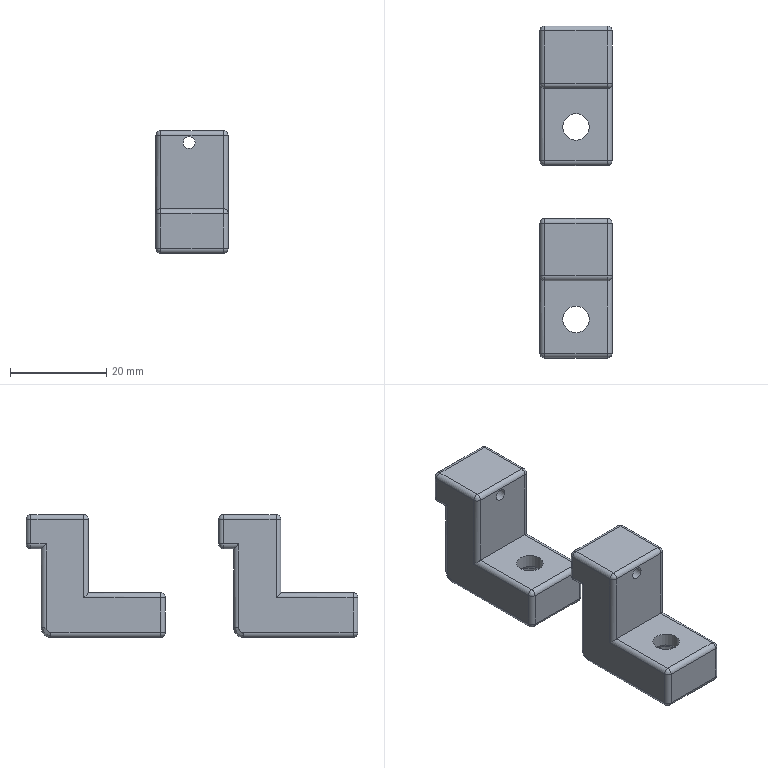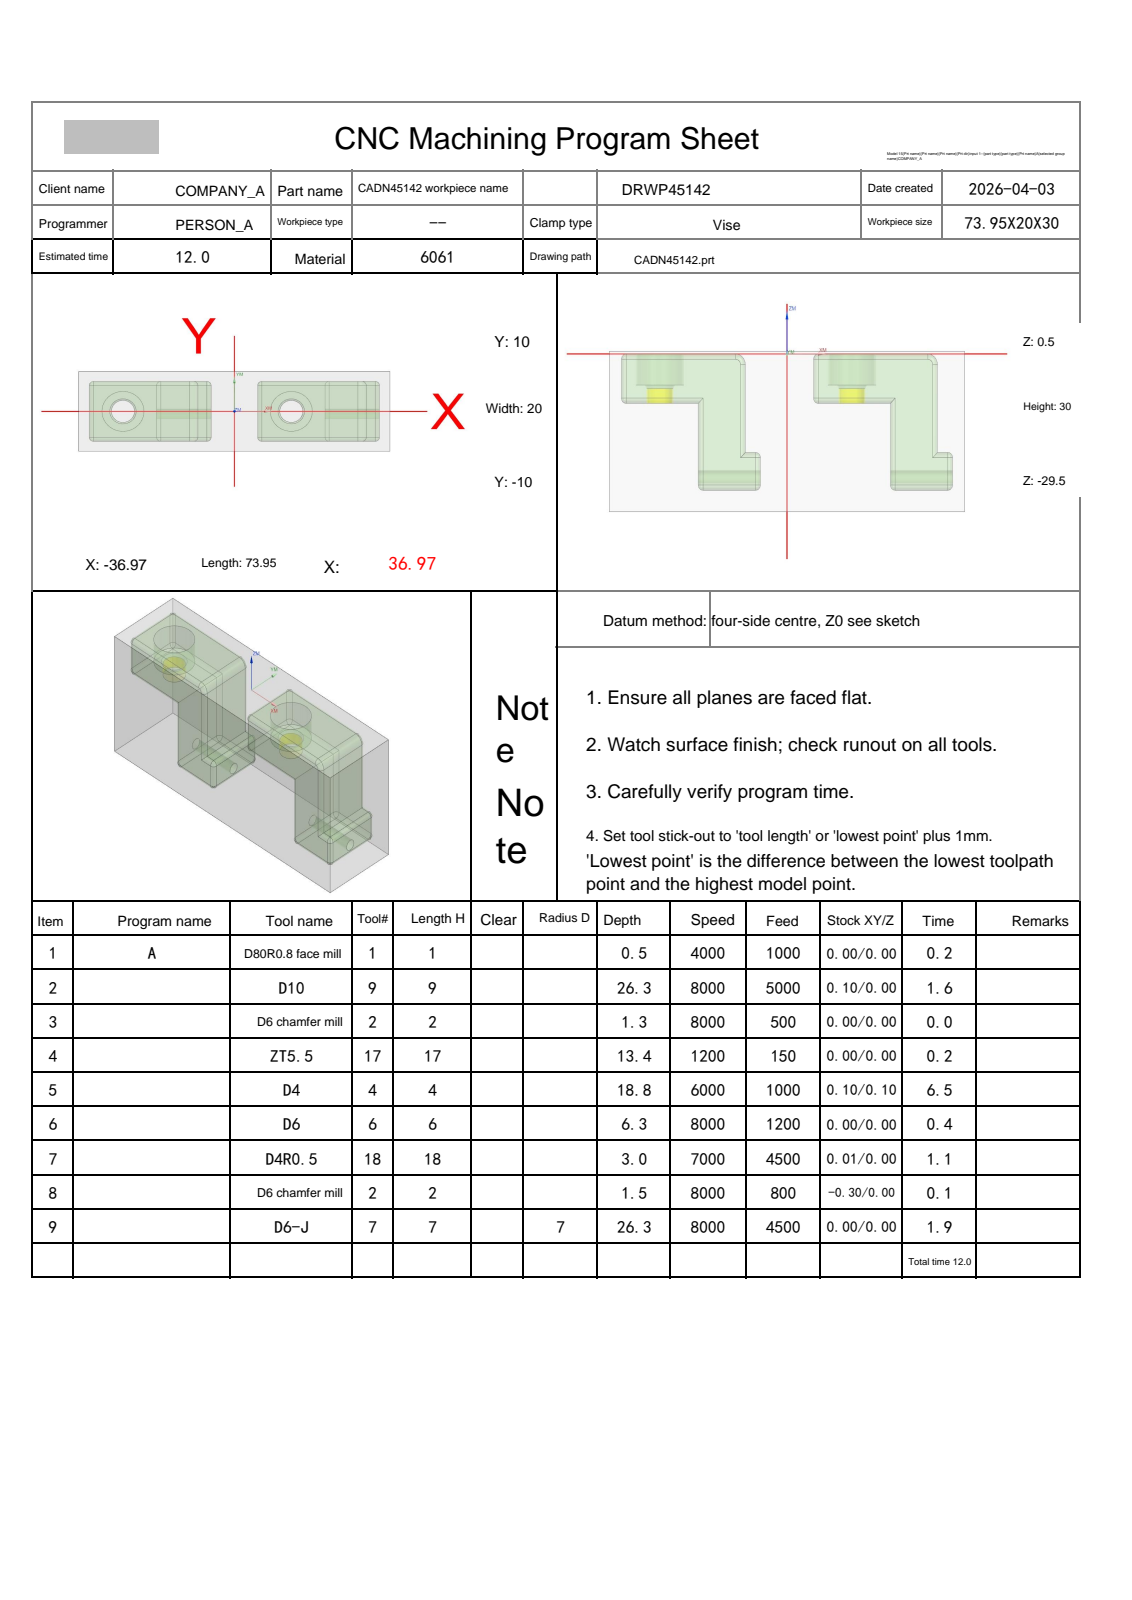NC program | NX | posted by the shop | part box 15 x 68.95 x 25.5 mm
Lines 4665 to 6074 of 6074:
N9 T07 M06
(D6-J  D=6. R=0. H=07 ce=0.00 di=0.00)
G00 G90 G54 X-34.389 Y11.516 M03 S8000
G43 H07 Z5.5
M08
Z-8.207
G01 Z-9.207 F1000.
G41 D07
X-34.371 Y11.317
G03 X-33.475 Y10.5 I.896 J.083
G01 X-9.675
X-9.386 Y10.489
G02 X-5.778 Y7.404 I-.289 J-3.99
X-5.675 Y6.5 I-3.896 J-.904
G01 X-5.674 Y-6.5
G02 X-5.736 Y-7.2 I-4. J0.0
X-9.674 Y-10.5 I-3.938 J.7
G01 X-33.475
G02 X-37.475 Y-6.5 I0.0 J4.
G01 Y6.5
G02 X-33.475 Y10.5 I4. J0.0
G03 X-32.575 Y11.4 I0.0 J.9
G01 G40 Y11.6
Z-8.207
G00 X-34.389 Y11.516
Z-17.413
G01 Z-18.413
G41 D07
X-34.371 Y11.317
G03 X-33.475 Y10.5 I.896 J.083
G01 X-9.675
G02 X-5.675 Y6.5 I0.0 J-4.
G01 X-5.674 Y-6.5
G02 X-9.674 Y-10.5 I-4. J0.0
G01 X-33.475
G02 X-37.475 Y-6.5 I0.0 J4.
G01 Y6.5
G02 X-33.475 Y10.5 I4. J0.0
G03 X-32.575 Y11.4 I0.0 J.9
G01 G40 Y11.6
Z-17.413
G00 Z5.5
X5.611 Y11.516
Z-8.207
G01 Z-9.207
G41 D07
X5.629 Y11.317
G03 X6.525 Y10.5 I.896 J.083
G01 X30.325
G02 X34.273 Y7.147 I0.0 J-4.
X34.325 Y6.5 I-3.947 J-.647
G01 X34.326 Y-6.5
G02 X30.326 Y-10.5 I-4. J0.0
G01 X6.525
G02 X2.525 Y-6.5 I0.0 J4.
G01 Y6.5
G02 X6.525 Y10.5 I4. J0.0
G03 X7.425 Y11.4 I0.0 J.9
G01 G40 Y11.6
Z-8.207
G00 X5.611 Y11.516
Z-17.413
G01 Z-18.413
G41 D07
X5.629 Y11.317
G03 X6.525 Y10.5 I.896 J.083
G01 X30.325
G02 X34.325 Y6.5 I0.0 J-4.
G01 X34.326 Y-6.5
G02 X30.326 Y-10.5 I-4. J0.0
G01 X6.525
G02 X2.525 Y-6.5 I0.0 J4.
G01 Y6.5
G02 X6.525 Y10.5 I4. J0.0
G03 X7.425 Y11.4 I0.0 J.9
G01 G40 Y11.6
Z-17.413
G00 Z5.5
G00 G90 X32.554 Y11.209 M03 S7000
Z10.5
Z-17.921
G01 Z-18.421 F4500.
G03 X32.372 Y10.575 I1.018 J-.635
X32.824 Y9.636 I1.2 J0.0
G01 X33.475
G02 X36.611 Y6.5 I0.0 J-3.136
G01 Y-6.5
G02 X33.475 Y-9.636 I-3.136 J0.0
G01 X32.825
X32.789 Y-9.664 Z-18.425
X33.475
G03 X36.639 Y-6.5 I0.0 J3.164
G01 Y6.5
G03 X33.475 Y9.664 I-3.164 J0.0
G01 X32.788
X32.758 Y9.688 Z-18.429
X33.475
G02 X36.663 Y6.5 I0.0 J-3.188
G01 Y-6.5
G02 X33.475 Y-9.688 I-3.188 J0.0
G01 X32.758
X32.73 Y-9.709 Z-18.433
X33.475
G03 X36.684 Y-6.5 I0.0 J3.209
G01 Y6.5
G03 X33.475 Y9.709 I-3.209 J0.0
G01 X32.73
X32.705 Y9.728 Z-18.437
X33.475
G02 X36.703 Y6.5 I0.0 J-3.228
G01 Y-6.5
G02 X33.475 Y-9.728 I-3.228 J0.0
G01 X32.705
X32.682 Y-9.745 Z-18.441
X33.475
G03 X36.72 Y-6.5 I0.0 J3.245
G01 Y6.5
G03 X33.475 Y9.745 I-3.245 J0.0
G01 X32.681
X32.659 Y9.761 Z-18.445
X33.475
G02 X36.736 Y6.5 I0.0 J-3.261
G01 Y-6.5
G02 X33.475 Y-9.761 I-3.261 J0.0
G01 X32.66
X32.638 Y-9.776 Z-18.449
X33.475
G03 X36.751 Y-6.5 I0.0 J3.277
G01 Y6.5
G03 X33.475 Y9.776 I-3.277 J0.0
G01 X32.637
X32.616 Y9.791 Z-18.454
X33.475
G02 X36.766 Y6.5 I0.0 J-3.292
G01 Y-6.5
G02 X33.475 Y-9.791 I-3.292 J0.0
G01 X32.616
X32.594 Y-9.807 Z-18.458
X33.475
G03 X36.782 Y-6.5 I0.0 J3.307
G01 Y6.5
G03 X33.475 Y9.807 I-3.307 J0.0
G01 X32.594
X32.574 Y9.82 Z-18.463
X33.475
G02 X36.795 Y6.5 I0.0 J-3.32
G01 Y-6.5
G02 X33.475 Y-9.82 I-3.32 J0.0
G01 X32.574
Z-18.468
X33.475
G03 X36.795 Y-6.5 I0.0 J3.32
G01 Y6.5
G03 X33.475 Y9.82 I-3.32 J0.0
G01 X32.574
X32.528 Y9.851 Z-18.473
X33.475
G02 X36.826 Y6.5 I0.0 J-3.351
G01 Y-6.5
G02 X33.475 Y-9.851 I-3.351 J0.0
G01 X32.528
X32.518 Y-9.858 Z-18.479
X33.475
G03 X36.833 Y-6.5 I0.0 J3.358
G01 Y6.5
G03 X33.475 Y9.858 I-3.358 J0.0
G01 X32.517
Z-18.484
X33.475
G02 X36.833 Y6.5 I0.0 J-3.358
G01 Y-6.5
G02 X33.475 Y-9.858 I-3.358 J0.0
G01 X32.518
X32.46 Y-9.895 Z-18.49
X33.475
G03 X36.869 Y-6.5 I0.0 J3.395
G01 Y6.5
G03 X33.475 Y9.895 I-3.395 J0.0
G01 X32.46
X32.437 Y9.909 Z-18.496
X33.475
G02 X36.884 Y6.5 I0.0 J-3.409
G01 Y-6.5
G02 X33.475 Y-9.909 I-3.409 J0.0
G01 X32.438
X32.415 Y-9.923 Z-18.502
X33.475
G03 X36.898 Y-6.5 I0.0 J3.423
G01 Y6.5
G03 X33.475 Y9.923 I-3.423 J0.0
G01 X32.414
X32.391 Y9.937 Z-18.509
X33.475
G02 X36.912 Y6.5 I0.0 J-3.437
G01 Y-6.5
G02 X33.475 Y-9.937 I-3.437 J0.0
G01 X32.392
X32.368 Y-9.951 Z-18.516
X33.475
G03 X36.926 Y-6.5 I0.0 J3.451
G01 Y6.5
G03 X33.475 Y9.951 I-3.451 J0.0
G01 X32.368
X32.345 Y9.964 Z-18.522
X33.475
G02 X36.939 Y6.5 I0.0 J-3.464
G01 Y-6.5
G02 X33.475 Y-9.964 I-3.464 J0.0
G01 X32.345
X32.322 Y-9.978 Z-18.529
X33.475
G03 X36.953 Y-6.5 I0.0 J3.478
G01 Y6.5
G03 X33.475 Y9.978 I-3.478 J0.0
G01 X32.321
X32.298 Y9.991 Z-18.537
X33.475
G02 X36.966 Y6.5 I0.0 J-3.491
G01 Y-6.5
G02 X33.475 Y-9.991 I-3.491 J0.0
G01 X32.298
X32.274 Y-10.005 Z-18.544
X33.475
G03 X36.98 Y-6.5 I0.0 J3.505
G01 Y6.5
G03 X33.475 Y10.005 I-3.505 J0.0
G01 X32.274
X32.25 Y10.018 Z-18.552
X33.475
G02 X36.993 Y6.5 I0.0 J-3.518
G01 Y-6.5
G02 X33.475 Y-10.018 I-3.518 J0.0
G01 X32.25
X32.226 Y-10.031 Z-18.56
X33.475
G03 X37.006 Y-6.5 I0.0 J3.531
G01 Y6.5
G03 X33.475 Y10.031 I-3.531 J0.0
G01 X32.226
X32.202 Y10.044 Z-18.568
X33.475
G02 X37.019 Y6.5 I0.0 J-3.544
G01 Y-6.5
G02 X33.475 Y-10.044 I-3.544 J0.0
G01 X32.202
X32.178 Y-10.057 Z-18.576
X33.475
G03 X37.032 Y-6.5 I0.0 J3.557
G01 Y6.5
G03 X33.475 Y10.057 I-3.557 J0.0
G01 X32.177
X32.153 Y10.069 Z-18.584
X33.475
G02 X37.044 Y6.5 I0.0 J-3.569
G01 Y-6.5
G02 X33.475 Y-10.069 I-3.569 J0.0
G01 X32.153
X32.128 Y-10.082 Z-18.593
X33.475
G03 X37.057 Y-6.5 I0.0 J3.582
G01 Y6.5
G03 X33.475 Y10.082 I-3.582 J0.0
G01 X32.128
X32.103 Y10.094 Z-18.602
X33.475
G02 X37.069 Y6.5 I0.0 J-3.594
G01 Y-6.5
G02 X33.475 Y-10.094 I-3.594 J0.0
G01 X32.104
X32.079 Y-10.106 Z-18.611
X33.475
G03 X37.081 Y-6.5 I0.0 J3.607
G01 Y6.5
G03 X33.475 Y10.106 I-3.607 J0.0
G01 X32.078
X32.053 Y10.119 Z-18.62
X33.475
G02 X37.093 Y6.5 I0.0 J-3.619
G01 Y-6.5
G02 X33.475 Y-10.119 I-3.619 J0.0
G01 X32.054
X32.028 Y-10.131 Z-18.629
X33.475
G03 X37.105 Y-6.5 I0.0 J3.631
G01 Y6.5
G03 X33.475 Y10.131 I-3.631 J0.0
G01 X32.028
X32.003 Y10.142 Z-18.639
X33.475
G02 X37.117 Y6.5 I0.0 J-3.642
G01 Y-6.5
G02 X33.475 Y-10.142 I-3.642 J0.0
G01 X32.003
X31.977 Y-10.154 Z-18.648
X33.475
G03 X37.129 Y-6.5 I0.0 J3.654
G01 Y6.5
G03 X33.475 Y10.154 I-3.654 J0.0
G01 X31.977
X31.951 Y10.165 Z-18.658
X33.475
G02 X37.14 Y6.5 I0.0 J-3.666
G01 Y-6.5
G02 X33.475 Y-10.165 I-3.666 J0.0
G01 X31.952
X31.926 Y-10.177 Z-18.668
X33.475
G03 X37.152 Y-6.5 I0.0 J3.677
G01 Y6.5
G03 X33.475 Y10.177 I-3.677 J0.0
G01 X31.925
X31.9 Y10.188 Z-18.678
X33.475
G02 X37.163 Y6.5 I0.0 J-3.688
G01 Y-6.5
G02 X33.475 Y-10.188 I-3.688 J0.0
G01 X31.9
X31.874 Y-10.199 Z-18.689
X33.475
G03 X37.174 Y-6.5 I0.0 J3.699
G01 Y6.5
G03 X33.475 Y10.199 I-3.699 J0.0
G01 X31.873
X31.847 Y10.21 Z-18.699
X33.475
G02 X37.185 Y6.5 I0.0 J-3.71
G01 Y-6.5
G02 X33.475 Y-10.21 I-3.71 J0.0
G01 X31.848
X31.821 Y-10.221 Z-18.71
X33.475
G03 X37.195 Y-6.5 I0.0 J3.721
G01 Y6.5
G03 X33.475 Y10.221 I-3.721 J0.0
G01 X31.821
X31.794 Y10.231 Z-18.72
X33.475
G02 X37.206 Y6.5 I0.0 J-3.731
G01 Y-6.5
G02 X33.475 Y-10.231 I-3.731 J0.0
G01 X31.795
X31.768 Y-10.242 Z-18.731
X33.475
G03 X37.216 Y-6.5 I0.0 J3.742
G01 Y6.5
G03 X33.475 Y10.242 I-3.742 J0.0
G01 X31.768
X31.741 Y10.252 Z-18.743
X33.475
G02 X37.227 Y6.5 I0.0 J-3.752
G01 Y-6.5
G02 X33.475 Y-10.252 I-3.752 J0.0
G01 X31.741
X31.714 Y-10.262 Z-18.754
X33.475
G03 X37.237 Y-6.5 I0.0 J3.762
G01 Y6.5
G03 X33.475 Y10.262 I-3.762 J0.0
G01 X31.714
X31.687 Y10.272 Z-18.765
X33.475
G02 X37.247 Y6.5 I0.0 J-3.772
G01 Y-6.5
G02 X33.475 Y-10.272 I-3.772 J0.0
G01 X31.687
X31.66 Y-10.281 Z-18.777
X33.475
G03 X37.256 Y-6.5 I0.0 J3.781
G01 Y6.5
G03 X33.475 Y10.281 I-3.781 J0.0
G01 X31.66
X31.633 Y10.291 Z-18.789
X33.475
G02 X37.266 Y6.5 I0.0 J-3.791
G01 Y-6.5
G02 X33.475 Y-10.291 I-3.791 J0.0
G01 X31.633
X31.606 Y-10.3 Z-18.8
X33.475
G03 X37.275 Y-6.5 I0.0 J3.8
G01 Y6.5
G03 X33.475 Y10.3 I-3.8 J0.0
G01 X31.605
X31.578 Y10.309 Z-18.812
X33.475
G02 X37.284 Y6.5 I0.0 J-3.809
G01 Y-6.5
G02 X33.475 Y-10.309 I-3.809 J0.0
G01 X31.578
X31.551 Y-10.318 Z-18.824
X33.475
G03 X37.293 Y-6.5 I0.0 J3.818
G01 Y6.5
G03 X33.475 Y10.318 I-3.818 J0.0
G01 X31.55
X31.523 Y10.327 Z-18.837
X33.475
G02 X37.302 Y6.5 I0.0 J-3.827
G01 Y-6.5
G02 X33.475 Y-10.327 I-3.827 J0.0
G01 X31.523
X31.495 Y-10.336 Z-18.849
X33.475
G03 X37.31 Y-6.5 I0.0 J3.836
G01 Y6.5
G03 X33.475 Y10.336 I-3.836 J0.0
G01 X31.495
X31.467 Y10.344 Z-18.862
X33.475
G02 X37.319 Y6.5 I0.0 J-3.844
G01 Y-6.5
G02 X33.475 Y-10.344 I-3.844 J0.0
G01 X31.467
X31.439 Y-10.352 Z-18.874
X33.475
G03 X37.327 Y-6.5 I0.0 J3.852
G01 Y6.5
G03 X33.475 Y10.352 I-3.852 J0.0
G01 X31.439
X31.411 Y10.36 Z-18.887
X33.475
G02 X37.335 Y6.5 I0.0 J-3.86
G01 Y-6.5
G02 X33.475 Y-10.36 I-3.86 J0.0
G01 X31.411
X31.383 Y-10.368 Z-18.9
X33.475
G03 X37.343 Y-6.5 I0.0 J3.868
G01 Y6.5
G03 X33.475 Y10.368 I-3.868 J0.0
G01 X31.382
X31.354 Y10.376 Z-18.913
X33.475
G02 X37.351 Y6.5 I0.0 J-3.876
G01 Y-6.5
G02 X33.475 Y-10.376 I-3.876 J0.0
G01 X31.354
X31.326 Y-10.383 Z-18.926
X33.475
G03 X37.358 Y-6.5 I0.0 J3.883
G01 Y6.5
G03 X33.475 Y10.383 I-3.883 J0.0
G01 X31.326
X31.297 Y10.39 Z-18.939
X33.475
G02 X37.365 Y6.5 I0.0 J-3.89
G01 Y-6.5
G02 X33.475 Y-10.39 I-3.89 J0.0
G01 X31.298
X31.269 Y-10.397 Z-18.952
X33.475
G03 X37.372 Y-6.5 I0.0 J3.898
G01 Y6.5
G03 X33.475 Y10.397 I-3.898 J0.0
G01 X31.269
X31.24 Y10.404 Z-18.966
X33.475
G02 X37.379 Y6.5 I0.0 J-3.904
G01 Y-6.5
G02 X33.475 Y-10.404 I-3.904 J0.0
G01 X31.24
X31.211 Y-10.411 Z-18.979
X33.475
G03 X37.386 Y-6.5 I0.0 J3.911
G01 Y6.5
G03 X33.475 Y10.411 I-3.911 J0.0
G01 X31.211
X31.182 Y10.417 Z-18.993
X33.475
G02 X37.392 Y6.5 I0.0 J-3.917
G01 Y-6.5
G02 X33.475 Y-10.417 I-3.917 J0.0
G01 X31.183
X31.154 Y-10.423 Z-19.007
X33.475
G03 X37.398 Y-6.5 I0.0 J3.924
G01 Y6.5
G03 X33.475 Y10.423 I-3.924 J0.0
G01 X31.153
X31.124 Y10.429 Z-19.02
X33.475
G02 X37.404 Y6.5 I0.0 J-3.93
G01 Y-6.5
G02 X33.475 Y-10.429 I-3.93 J0.0
G01 X31.125
X31.096 Y-10.435 Z-19.034
X33.475
G03 X37.41 Y-6.5 I0.0 J3.935
G01 Y6.5
G03 X33.475 Y10.435 I-3.935 J0.0
G01 X31.095
X31.066 Y10.441 Z-19.048
X33.475
G02 X37.416 Y6.5 I0.0 J-3.941
G01 Y-6.5
G02 X33.475 Y-10.441 I-3.941 J0.0
G01 X31.066
X31.037 Y-10.446 Z-19.062
X33.475
G03 X37.421 Y-6.5 I0.0 J3.946
G01 Y6.5
G03 X33.475 Y10.446 I-3.946 J0.0
G01 X31.037
X31.008 Y10.451 Z-19.076
X33.475
G02 X37.426 Y6.5 I0.0 J-3.952
G01 Y-6.5
G02 X33.475 Y-10.451 I-3.952 J0.0
G01 X31.008
X30.979 Y-10.456 Z-19.09
X33.475
G03 X37.431 Y-6.5 I0.0 J3.957
G01 Y6.5
G03 X33.475 Y10.456 I-3.957 J0.0
G01 X30.978
X30.949 Y10.461 Z-19.105
X33.475
G02 X37.436 Y6.5 I0.0 J-3.961
G01 Y-6.5
G02 X33.475 Y-10.461 I-3.961 J0.0
G01 X30.949
X30.92 Y-10.466 Z-19.119
X33.475
G03 X37.441 Y-6.5 I0.0 J3.966
G01 Y6.5
G03 X33.475 Y10.466 I-3.966 J0.0
G01 X30.919
X30.89 Y10.47 Z-19.133
X33.475
G02 X37.445 Y6.5 I0.0 J-3.97
G01 Y-6.5
G02 X33.475 Y-10.47 I-3.97 J0.0
G01 X30.89
X30.861 Y-10.474 Z-19.148
X33.475
G03 X37.449 Y-6.5 I0.0 J3.974
G01 Y6.5
G03 X33.475 Y10.474 I-3.974 J0.0
G01 X30.86
X30.831 Y10.478 Z-19.162
X33.475
G02 X37.453 Y6.5 I0.0 J-3.978
G01 Y-6.5
G02 X33.475 Y-10.478 I-3.978 J0.0
G01 X30.831
X30.801 Y-10.482 Z-19.177
X33.475
G03 X37.456 Y-6.5 I0.0 J3.982
G01 Y6.5
G03 X33.475 Y10.482 I-3.982 J0.0
G01 X30.801
X30.771 Y10.485 Z-19.192
X33.475
G02 X37.46 Y6.5 I0.0 J-3.985
G01 Y-6.5
G02 X33.475 Y-10.485 I-3.985 J0.0
G01 X30.771
X30.742 Y-10.488 Z-19.206
X33.475
G03 X37.463 Y-6.5 I0.0 J3.988
G01 Y6.5
G03 X33.475 Y10.488 I-3.988 J0.0
G01 X30.741
X30.629 Y10.498 Z-19.214
X30.516 Y10.491 Z-19.221
X33.475
G02 X37.466 Y6.5 I0.0 J-3.991
G01 Y-6.5
G02 X33.475 Y-10.491 I-3.991 J0.0
G01 X30.516
X30.501 Y-10.494 Z-19.236
X33.475
G03 X37.469 Y-6.5 I0.0 J3.994
G01 Y6.5
G03 X33.475 Y10.494 I-3.994 J0.0
G01 X30.501
X30.487 Y10.497 Z-19.251
X33.475
G02 X37.471 Y6.5 I0.0 J-3.997
G01 Y-6.5
G02 X33.475 Y-10.497 I-3.997 J0.0
G01 X30.487
X30.472 Y-10.499 Z-19.265
X33.475
G03 X37.474 Y-6.5 I0.0 J3.999
G01 Y6.5
G03 X33.475 Y10.499 I-3.999 J0.0
G01 X30.472
X30.457 Y10.501 Z-19.28
X33.475
G02 X37.476 Y6.5 I0.0 J-4.001
G01 Y-6.5
G02 X33.475 Y-10.501 I-4.001 J0.0
G01 X30.458
X30.342 Y-10.51 Z-19.288
X30.226 Z-19.295
X30.443 Y-10.503
X33.475
G03 X37.478 Y-6.5 I0.0 J4.003
G01 Y6.5
G03 X33.475 Y10.503 I-4.003 J0.0
G01 X30.443
X30.428 Y10.505 Z-19.31
X33.475
G02 X37.479 Y6.5 I0.0 J-4.005
G01 Y-6.5
G02 X33.475 Y-10.505 I-4.005 J0.0
G01 X30.428
X30.226 Y-10.51
Z-19.325
X30.413 Y-10.506
X33.475
G03 X37.481 Y-6.5 I0.0 J4.006
G01 Y6.5
G03 X33.475 Y10.506 I-4.006 J0.0
G01 X30.413
X30.377 Y10.509
X28.949
X28.798 Z-19.34
X30.377
X30.398 Y10.507
X33.475
G02 X37.482 Y6.5 I0.0 J-4.007
G01 Y-6.5
G02 X33.475 Y-10.507 I-4.007 J0.0
G01 X30.399
X30.226 Y-10.51
Z-19.355
X30.384 Y-10.508
X33.475
G03 X37.483 Y-6.5 I0.0 J4.008
G01 Y6.5
G03 X33.475 Y10.508 I-4.008 J0.0
G01 X30.383
X28.777 Y10.509
X28.755 Z-19.37
X30.377
X33.475
G02 X37.484 Y6.5 I0.0 J-4.009
G01 Y-6.5
X37.482 Y-6.625
G02 X33.475 Y-10.509 I-4.007 J.125
G01 X30.377
X30.226 Y-10.51
Z-19.385
X30.377 Y-10.509
X33.475
X33.587 Y-10.508
G03 X34.575 Y-10.356 I-.112 J4.008
G01 X34.72 Y-10.311
G03 X35.172 Y-10.133 I-1.246 J3.811
G01 X35.349 Y-10.045
G03 X35.677 Y-9.851 I-1.874 J3.545
G01 X35.808 Y-9.761
G03 X36.26 Y-9.384 I-2.333 J3.261
G01 X36.391 Y-9.251
G03 X36.741 Y-8.825 I-2.917 J2.751
G01 X36.895 Y-8.592
X36.93 Y-8.534
G03 X37.128 Y-8.152 I-3.455 J2.035
G01 X37.206 Y-7.968
G03 X37.482 Y-6.625 I-3.731 J1.468
G01 X37.484 Y-6.5
Y6.5
X37.482 Y6.625
G03 X37.078 Y8.258 I-4.008 J-.125
G01 X36.974 Y8.457
X36.954 Y8.492
G03 X36.79 Y8.756 I-3.48 J-1.992
G01 X36.741 Y8.825
G03 X36.391 Y9.251 I-3.266 J-2.325
G01 X36.26 Y9.384
G03 X35.808 Y9.761 I-2.785 J-2.884
G01 X35.643 Y9.873
G03 X35.358 Y10.04 I-2.168 J-3.373
G01 X35.275 Y10.082
X34.861 Y10.262
X34.72 Y10.311
X34.58 Y10.354
X34.46 Y10.386
X34.188 Y10.445
X34.117 Y10.458
X33.697 Y10.503
X33.587 Y10.508
X33.475 Y10.509
X30.377
X28.733
X28.712 Z-19.4
X30.377 Y10.51
X33.475
X33.61 Y10.508
X33.697 Y10.503
X34.117 Y10.458
X34.171 Y10.449
X34.46 Y10.387
X34.58 Y10.355
X34.695 Y10.319
X34.732 Y10.308
G02 X36.26 Y9.384 I-1.257 J-3.808
G01 X36.392 Y9.251
G02 X37.483 Y6.625 I-2.917 J-2.752
G01 X37.484 Y-6.5
X37.483 Y-6.625
G02 X37.271 Y-7.792 I-4.008 J.125
G01 X37.122 Y-8.165
X37.108 Y-8.197
G02 X36.93 Y-8.535 I-3.633 J1.698
G01 X36.895 Y-8.592
X36.741 Y-8.826
G02 X36.392 Y-9.251 I-3.267 J2.326
G01 X36.26 Y-9.384
G02 X34.72 Y-10.311 I-2.785 J2.885
G01 X34.695 Y-10.319
X34.575 Y-10.356
G02 X34.171 Y-10.449 I-1.1 J3.856
G01 X34.141 Y-10.454
G02 X33.598 Y-10.508 I-.666 J3.954
G01 X33.475 Y-10.51
X30.377
X30.226
Z-19.413
X33.546
X33.655 Y-10.506
G03 X34.141 Y-10.454 I-.18 J4.006
G01 X34.616 Y-10.345
G03 X35.832 Y-9.744 I-1.19 J3.941
X36.724 Y-8.85 I-2.358 J3.244
G01 X36.769 Y-8.787
G03 X37.483 Y-6.625 I-3.294 J2.287
G01 X37.484 Y-6.5
X37.483 Y6.625
G03 X36.392 Y9.251 I-4.008 J-.125
G01 X36.249 Y9.395
G03 X35.808 Y9.761 I-2.774 J-2.896
X34.732 Y10.308 I-2.373 J-3.337
G01 X34.579 Y10.354
X34.58 Y10.355
G03 X34.117 Y10.458 I-1.105 J-3.855
X33.546 Y10.51 I-.606 J-3.513
G01 X28.685
G00 Z10.5
X-7.446 Y11.209
Z-17.921
G01 Z-18.421
G03 X-7.628 Y10.575 I1.018 J-.635
X-7.176 Y9.636 I1.2 J0.0
G01 X-6.525
G02 X-3.389 Y6.5 I0.0 J-3.136
G01 Y-6.5
G02 X-6.525 Y-9.636 I-3.136 J0.0
G01 X-7.175
X-7.211 Y-9.664 Z-18.425
X-6.525
G03 X-3.361 Y-6.5 I0.0 J3.164
G01 Y6.5
G03 X-6.525 Y9.664 I-3.164 J0.0
G01 X-7.212
X-7.242 Y9.688 Z-18.429
X-6.525
G02 X-3.337 Y6.5 I0.0 J-3.188
G01 Y-6.5
G02 X-6.525 Y-9.688 I-3.188 J0.0
G01 X-7.242
X-7.27 Y-9.709 Z-18.433
X-6.525
G03 X-3.316 Y-6.5 I0.0 J3.209
G01 Y6.5
G03 X-6.525 Y9.709 I-3.209 J0.0
G01 X-7.27
X-7.295 Y9.728 Z-18.437
X-6.525
G02 X-3.297 Y6.5 I0.0 J-3.228
G01 Y-6.5
G02 X-6.525 Y-9.728 I-3.228 J0.0
G01 X-7.295
X-7.318 Y-9.745 Z-18.441
X-6.525
G03 X-3.28 Y-6.5 I0.0 J3.245
G01 Y6.5
G03 X-6.525 Y9.745 I-3.245 J0.0
G01 X-7.319
X-7.341 Y9.761 Z-18.445
X-6.525
G02 X-3.264 Y6.5 I0.0 J-3.261
G01 Y-6.5
G02 X-6.525 Y-9.761 I-3.261 J0.0
G01 X-7.34
X-7.362 Y-9.776 Z-18.449
X-6.525
G03 X-3.249 Y-6.5 I0.0 J3.277
G01 Y6.5
G03 X-6.525 Y9.776 I-3.277 J0.0
G01 X-7.363
X-7.384 Y9.791 Z-18.454
X-6.525
G02 X-3.234 Y6.5 I0.0 J-3.292
G01 Y-6.5
G02 X-6.525 Y-9.791 I-3.292 J0.0
G01 X-7.384
X-7.406 Y-9.807 Z-18.458
X-6.525
G03 X-3.218 Y-6.5 I0.0 J3.307
G01 Y6.5
G03 X-6.525 Y9.807 I-3.307 J0.0
G01 X-7.406
X-7.426 Y9.82 Z-18.463
X-6.525
G02 X-3.205 Y6.5 I0.0 J-3.32
G01 Y-6.5
G02 X-6.525 Y-9.82 I-3.32 J0.0
G01 X-7.426
Z-18.468
X-6.525
G03 X-3.205 Y-6.5 I0.0 J3.32
G01 Y6.5
G03 X-6.525 Y9.82 I-3.32 J0.0
G01 X-7.426
X-7.472 Y9.851 Z-18.473
X-6.525
G02 X-3.174 Y6.5 I0.0 J-3.351
G01 Y-6.5
G02 X-6.525 Y-9.851 I-3.351 J0.0
G01 X-7.472
X-7.482 Y-9.858 Z-18.479
X-6.525
G03 X-3.167 Y-6.5 I0.0 J3.358
G01 Y6.5
G03 X-6.525 Y9.858 I-3.358 J0.0
G01 X-7.483
Z-18.484
X-6.525
G02 X-3.167 Y6.5 I0.0 J-3.358
G01 Y-6.5
G02 X-6.525 Y-9.858 I-3.358 J0.0
G01 X-7.482
X-7.54 Y-9.895 Z-18.49
X-6.525
G03 X-3.131 Y-6.5 I0.0 J3.395
G01 Y6.5
G03 X-6.525 Y9.895 I-3.395 J0.0
G01 X-7.54
X-7.563 Y9.909 Z-18.496
X-6.525
G02 X-3.116 Y6.5 I0.0 J-3.409
G01 Y-6.5
G02 X-6.525 Y-9.909 I-3.409 J0.0
G01 X-7.562
X-7.585 Y-9.923 Z-18.502
X-6.525
G03 X-3.102 Y-6.5 I0.0 J3.423
G01 Y6.5
G03 X-6.525 Y9.923 I-3.423 J0.0
G01 X-7.586
X-7.609 Y9.937 Z-18.509
X-6.525
G02 X-3.088 Y6.5 I0.0 J-3.437
G01 Y-6.5
G02 X-6.525 Y-9.937 I-3.437 J0.0
G01 X-7.608
X-7.632 Y-9.951 Z-18.516
X-6.525
G03 X-3.074 Y-6.5 I0.0 J3.451
G01 Y6.5
G03 X-6.525 Y9.951 I-3.451 J0.0
G01 X-7.632
X-7.655 Y9.964 Z-18.522
X-6.525
G02 X-3.061 Y6.5 I0.0 J-3.464
G01 Y-6.5
G02 X-6.525 Y-9.964 I-3.464 J0.0
G01 X-7.655
X-7.678 Y-9.978 Z-18.529
X-6.525
G03 X-3.047 Y-6.5 I0.0 J3.478
G01 Y6.5
G03 X-6.525 Y9.978 I-3.478 J0.0
G01 X-7.679
X-7.702 Y9.991 Z-18.537
X-6.525
G02 X-3.034 Y6.5 I0.0 J-3.491
G01 Y-6.5
G02 X-6.525 Y-9.991 I-3.491 J0.0
G01 X-7.702
X-7.726 Y-10.005 Z-18.544
X-6.525
G03 X-3.02 Y-6.5 I0.0 J3.505
G01 Y6.5
G03 X-6.525 Y10.005 I-3.505 J0.0
G01 X-7.726
X-7.75 Y10.018 Z-18.552
X-6.525
G02 X-3.007 Y6.5 I0.0 J-3.518
G01 Y-6.5
G02 X-6.525 Y-10.018 I-3.518 J0.0
G01 X-7.75
X-7.774 Y-10.031 Z-18.56
X-6.525
G03 X-2.994 Y-6.5 I0.0 J3.531
G01 Y6.5
G03 X-6.525 Y10.031 I-3.531 J0.0
G01 X-7.774
X-7.798 Y10.044 Z-18.568
X-6.525
G02 X-2.981 Y6.5 I0.0 J-3.544
G01 Y-6.5
G02 X-6.525 Y-10.044 I-3.544 J0.0
G01 X-7.798
X-7.822 Y-10.057 Z-18.576
X-6.525
G03 X-2.968 Y-6.5 I0.0 J3.557
G01 Y6.5
G03 X-6.525 Y10.057 I-3.557 J0.0
G01 X-7.823
X-7.847 Y10.069 Z-18.584
X-6.525
G02 X-2.956 Y6.5 I0.0 J-3.569
G01 Y-6.5
G02 X-6.525 Y-10.069 I-3.569 J0.0
G01 X-7.847
X-7.872 Y-10.082 Z-18.593
X-6.525
G03 X-2.943 Y-6.5 I0.0 J3.582
G01 Y6.5
G03 X-6.525 Y10.082 I-3.582 J0.0
G01 X-7.872
X-7.897 Y10.094 Z-18.602
X-6.525
G02 X-2.931 Y6.5 I0.0 J-3.594
G01 Y-6.5
G02 X-6.525 Y-10.094 I-3.594 J0.0
G01 X-7.896
X-7.921 Y-10.106 Z-18.611
X-6.525
G03 X-2.919 Y-6.5 I0.0 J3.607
G01 Y6.5
G03 X-6.525 Y10.106 I-3.607 J0.0
G01 X-7.922
X-7.947 Y10.119 Z-18.62
X-6.525
G02 X-2.907 Y6.5 I0.0 J-3.619
G01 Y-6.5
G02 X-6.525 Y-10.119 I-3.619 J0.0
G01 X-7.946
X-7.972 Y-10.131 Z-18.629
X-6.525
G03 X-2.895 Y-6.5 I0.0 J3.631
G01 Y6.5
G03 X-6.525 Y10.131 I-3.631 J0.0
G01 X-7.972
X-7.997 Y10.142 Z-18.639
X-6.525
G02 X-2.883 Y6.5 I0.0 J-3.642
G01 Y-6.5
G02 X-6.525 Y-10.142 I-3.642 J0.0
G01 X-7.997
X-8.023 Y-10.154 Z-18.648
X-6.525
G03 X-2.871 Y-6.5 I0.0 J3.654
G01 Y6.5
G03 X-6.525 Y10.154 I-3.654 J0.0
G01 X-8.023
X-8.049 Y10.165 Z-18.658
X-6.525
G02 X-2.86 Y6.5 I0.0 J-3.666
G01 Y-6.5
G02 X-6.525 Y-10.165 I-3.666 J0.0
G01 X-8.048
X-8.074 Y-10.177 Z-18.668
X-6.525
G03 X-2.848 Y-6.5 I0.0 J3.677
G01 Y6.5
G03 X-6.525 Y10.177 I-3.677 J0.0
G01 X-8.075
X-8.1 Y10.188 Z-18.678
X-6.525
G02 X-2.837 Y6.5 I0.0 J-3.688
G01 Y-6.5
G02 X-6.525 Y-10.188 I-3.688 J0.0
G01 X-8.1
X-8.126 Y-10.199 Z-18.689
X-6.525
G03 X-2.826 Y-6.5 I0.0 J3.699
G01 Y6.5
G03 X-6.525 Y10.199 I-3.699 J0.0
G01 X-8.127
X-8.153 Y10.21 Z-18.699
X-6.525
G02 X-2.815 Y6.5 I0.0 J-3.71
G01 Y-6.5
G02 X-6.525 Y-10.21 I-3.71 J0.0
G01 X-8.152
X-8.179 Y-10.221 Z-18.71
X-6.525
G03 X-2.805 Y-6.5 I0.0 J3.721
G01 Y6.5
G03 X-6.525 Y10.221 I-3.721 J0.0
G01 X-8.179
X-8.206 Y10.231 Z-18.72
X-6.525
G02 X-2.794 Y6.5 I0.0 J-3.731
G01 Y-6.5
G02 X-6.525 Y-10.231 I-3.731 J0.0
G01 X-8.205
X-8.232 Y-10.242 Z-18.731
X-6.525
G03 X-2.784 Y-6.5 I0.0 J3.742
G01 Y6.5
G03 X-6.525 Y10.242 I-3.742 J0.0
G01 X-8.232
X-8.259 Y10.252 Z-18.743
X-6.525
G02 X-2.773 Y6.5 I0.0 J-3.752
G01 Y-6.5
G02 X-6.525 Y-10.252 I-3.752 J0.0
G01 X-8.259
X-8.286 Y-10.262 Z-18.754
X-6.525
G03 X-2.763 Y-6.5 I0.0 J3.762
G01 Y6.5
G03 X-6.525 Y10.262 I-3.762 J0.0
G01 X-8.286
X-8.313 Y10.272 Z-18.765
X-6.525
G02 X-2.753 Y6.5 I0.0 J-3.772
G01 Y-6.5
G02 X-6.525 Y-10.272 I-3.772 J0.0
G01 X-8.313
X-8.34 Y-10.281 Z-18.777
X-6.525
G03 X-2.744 Y-6.5 I0.0 J3.781
G01 Y6.5
G03 X-6.525 Y10.281 I-3.781 J0.0
G01 X-8.34
X-8.367 Y10.291 Z-18.789
X-6.525
G02 X-2.734 Y6.5 I0.0 J-3.791
G01 Y-6.5
G02 X-6.525 Y-10.291 I-3.791 J0.0
G01 X-8.367
X-8.394 Y-10.3 Z-18.8
X-6.525
G03 X-2.725 Y-6.5 I0.0 J3.8
G01 Y6.5
G03 X-6.525 Y10.3 I-3.8 J0.0
G01 X-8.395
X-8.422 Y10.309 Z-18.812
X-6.525
G02 X-2.716 Y6.5 I0.0 J-3.809
G01 Y-6.5
G02 X-6.525 Y-10.309 I-3.809 J0.0
G01 X-8.422
X-8.449 Y-10.318 Z-18.824
X-6.525
G03 X-2.707 Y-6.5 I0.0 J3.818
G01 Y6.5
G03 X-6.525 Y10.318 I-3.818 J0.0
G01 X-8.45
X-8.477 Y10.327 Z-18.837
X-6.525
G02 X-2.698 Y6.5 I0.0 J-3.827
G01 Y-6.5
G02 X-6.525 Y-10.327 I-3.827 J0.0
G01 X-8.477
X-8.505 Y-10.336 Z-18.849
X-6.525
G03 X-2.69 Y-6.5 I0.0 J3.836
G01 Y6.5
G03 X-6.525 Y10.336 I-3.836 J0.0
G01 X-8.505
X-8.533 Y10.344 Z-18.862
X-6.525
G02 X-2.681 Y6.5 I0.0 J-3.844
G01 Y-6.5
G02 X-6.525 Y-10.344 I-3.844 J0.0
G01 X-8.533
X-8.561 Y-10.352 Z-18.874
X-6.525
G03 X-2.673 Y-6.5 I0.0 J3.852
G01 Y6.5
G03 X-6.525 Y10.352 I-3.852 J0.0
G01 X-8.561
X-8.589 Y10.36 Z-18.887
X-6.525
G02 X-2.665 Y6.5 I0.0 J-3.86
G01 Y-6.5
G02 X-6.525 Y-10.36 I-3.86 J0.0
G01 X-8.589
X-8.617 Y-10.368 Z-18.9
X-6.525
G03 X-2.657 Y-6.5 I0.0 J3.868
G01 Y6.5
G03 X-6.525 Y10.368 I-3.868 J0.0
G01 X-8.618
X-8.646 Y10.376 Z-18.913
X-6.525
G02 X-2.649 Y6.5 I0.0 J-3.876
G01 Y-6.5
G02 X-6.525 Y-10.376 I-3.876 J0.0
G01 X-8.646
X-8.674 Y-10.383 Z-18.926
X-6.525
G03 X-2.642 Y-6.5 I0.0 J3.883
G01 Y6.5
G03 X-6.525 Y10.383 I-3.883 J0.0
G01 X-8.674
X-8.703 Y10.39 Z-18.939
X-6.525
G02 X-2.635 Y6.5 I0.0 J-3.89
G01 Y-6.5
G02 X-6.525 Y-10.39 I-3.89 J0.0
G01 X-8.702
X-8.731 Y-10.397 Z-18.952
X-6.525
G03 X-2.628 Y-6.5 I0.0 J3.898
G01 Y6.5
G03 X-6.525 Y10.397 I-3.898 J0.0
G01 X-8.731
X-8.76 Y10.404 Z-18.966
X-6.525
G02 X-2.621 Y6.5 I0.0 J-3.904
G01 Y-6.5
G02 X-6.525 Y-10.404 I-3.904 J0.0
G01 X-8.76
X-8.789 Y-10.411 Z-18.979
X-6.525
G03 X-2.614 Y-6.5 I0.0 J3.911
G01 Y6.5
G03 X-6.525 Y10.411 I-3.911 J0.0
G01 X-8.789
X-8.818 Y10.417 Z-18.993
X-6.525
G02 X-2.608 Y6.5 I0.0 J-3.917
G01 Y-6.5
G02 X-6.525 Y-10.417 I-3.917 J0.0
G01 X-8.817
X-8.846 Y-10.423 Z-19.007
X-6.525
G03 X-2.602 Y-6.5 I0.0 J3.924
G01 Y6.5
G03 X-6.525 Y10.423 I-3.924 J0.0
G01 X-8.847
X-8.876 Y10.429 Z-19.02
X-6.525
G02 X-2.596 Y6.5 I0.0 J-3.93
G01 Y-6.5
G02 X-6.525 Y-10.429 I-3.93 J0.0
G01 X-8.875
X-8.904 Y-10.435 Z-19.034
X-6.525
G03 X-2.59 Y-6.5 I0.0 J3.935
G01 Y6.5
G03 X-6.525 Y10.435 I-3.935 J0.0
G01 X-8.905
X-8.934 Y10.441 Z-19.048
X-6.525
G02 X-2.584 Y6.5 I0.0 J-3.941
G01 Y-6.5
G02 X-6.525 Y-10.441 I-3.941 J0.0
G01 X-8.934
X-8.963 Y-10.446 Z-19.062
X-6.525
G03 X-2.579 Y-6.5 I0.0 J3.946
G01 Y6.5
G03 X-6.525 Y10.446 I-3.946 J0.0
G01 X-8.963
X-8.992 Y10.451 Z-19.076
X-6.525
G02 X-2.574 Y6.5 I0.0 J-3.952
G01 Y-6.5
G02 X-6.525 Y-10.451 I-3.952 J0.0
G01 X-8.992
X-9.021 Y-10.456 Z-19.09
X-6.525
G03 X-2.569 Y-6.5 I0.0 J3.957
G01 Y6.5
G03 X-6.525 Y10.456 I-3.957 J0.0
G01 X-9.022
X-9.051 Y10.461 Z-19.105
X-6.525
G02 X-2.564 Y6.5 I0.0 J-3.961
G01 Y-6.5
G02 X-6.525 Y-10.461 I-3.961 J0.0
G01 X-9.051
X-9.08 Y-10.466 Z-19.119
X-6.525
G03 X-2.559 Y-6.5 I0.0 J3.966
G01 Y6.5
G03 X-6.525 Y10.466 I-3.966 J0.0
G01 X-9.081
X-9.11 Y10.47 Z-19.133
X-6.525
G02 X-2.555 Y6.5 I0.0 J-3.97
G01 Y-6.5
G02 X-6.525 Y-10.47 I-3.97 J0.0
G01 X-9.11
X-9.139 Y-10.474 Z-19.148
X-6.525
G03 X-2.551 Y-6.5 I0.0 J3.974
G01 Y6.5
G03 X-6.525 Y10.474 I-3.974 J0.0
G01 X-9.14
X-9.169 Y10.478 Z-19.162
X-6.525
G02 X-2.547 Y6.5 I0.0 J-3.978
G01 Y-6.5
G02 X-6.525 Y-10.478 I-3.978 J0.0
G01 X-9.169
X-9.199 Y-10.482 Z-19.177
X-6.525
G03 X-2.544 Y-6.5 I0.0 J3.982
G01 Y6.5
G03 X-6.525 Y10.482 I-3.982 J0.0
G01 X-9.199
X-9.229 Y10.485 Z-19.192
X-6.525
G02 X-2.54 Y6.5 I0.0 J-3.985
G01 Y-6.5
G02 X-6.525 Y-10.485 I-3.985 J0.0
G01 X-9.229
X-9.258 Y-10.488 Z-19.206
X-6.525
G03 X-2.537 Y-6.5 I0.0 J3.988
G01 Y6.5
G03 X-6.525 Y10.488 I-3.988 J0.0
G01 X-9.259
X-9.288 Y10.491 Z-19.221
X-6.525
G02 X-2.534 Y6.5 I0.0 J-3.991
G01 Y-6.5
G02 X-6.525 Y-10.491 I-3.991 J0.0
G01 X-9.288
X-9.393 Y-10.5 Z-19.228
X-9.499 Y-10.494 Z-19.236
X-6.525
G03 X-2.531 Y-6.5 I0.0 J3.994
G01 Y6.5
G03 X-6.525 Y10.494 I-3.994 J0.0
G01 X-9.499
X-9.513 Y10.497 Z-19.251
X-6.525
G02 X-2.529 Y6.5 I0.0 J-3.997
G01 Y-6.5
G02 X-6.525 Y-10.497 I-3.997 J0.0
G01 X-9.513
X-9.528 Y-10.499 Z-19.265
X-6.525
G03 X-2.526 Y-6.5 I0.0 J3.999
G01 Y6.5
G03 X-6.525 Y10.499 I-3.999 J0.0
G01 X-9.528
X-9.543 Y10.501 Z-19.28
X-6.525
G02 X-2.524 Y6.5 I0.0 J-4.001
G01 Y-6.5
G02 X-6.525 Y-10.501 I-4.001 J0.0
G01 X-9.542
X-9.659 Y-10.51 Z-19.288
X-9.776 Z-19.295
X-9.557 Y-10.503
X-6.525
G03 X-2.522 Y-6.5 I0.0 J4.003
G01 Y6.5
G03 X-6.525 Y10.503 I-4.003 J0.0
G01 X-9.557
X-9.572 Y10.505 Z-19.31
X-6.525
G02 X-2.521 Y6.5 I0.0 J-4.005
G01 Y-6.5
G02 X-6.525 Y-10.505 I-4.005 J0.0
G01 X-9.572
X-9.776 Y-10.51
Z-19.325
X-9.587 Y-10.506
X-6.525
G03 X-2.519 Y-6.5 I0.0 J4.006
G01 Y6.5
G03 X-6.525 Y10.506 I-4.006 J0.0
G01 X-9.587
X-9.658 Y10.509
X-11.046
X-11.196 Z-19.34
X-9.658
X-9.602 Y10.507
X-6.525
G02 X-2.518 Y6.5 I0.0 J-4.007
G01 Y-6.5
G02 X-6.525 Y-10.507 I-4.007 J0.0
G01 X-9.601
X-9.776 Y-10.51
Z-19.355
X-9.616 Y-10.508
X-6.525
G03 X-2.517 Y-6.5 I0.0 J4.008
G01 Y6.5
G03 X-6.525 Y10.508 I-4.008 J0.0
G01 X-9.617
X-9.658 Y10.509
X-11.218
X-11.25 Z-19.37
X-9.632
X-6.525
G02 X-2.516 Y6.5 I0.0 J-4.009
G01 Y-6.51
G02 X-6.525 Y-10.509 I-4.009 J.01
G01 X-9.631
X-9.776 Y-10.51
Z-19.385
X-9.646 Y-10.509
X-6.525
X-6.41 Y-10.508
G03 X-5.272 Y-10.309 I-.116 J4.008
G01 X-5.208 Y-10.287
G03 X-3.02 Y-8.446 I-1.317 J3.787
G01 X-2.933 Y-8.281
G03 X-2.623 Y-7.421 I-3.592 J1.781
G01 X-2.581 Y-7.217
X-2.569 Y-7.151
G03 X-2.518 Y-6.628 I-3.956 J.651
G01 X-2.516 Y-6.53
Y6.53
X-2.518 Y6.64
G03 X-6.41 Y10.508 I-4.007 J-.14
G01 X-6.525 Y10.509
X-9.646
X-11.271
X-11.293 Z-19.4
X-9.658 Y10.51
X-6.525
X-6.319 Y10.505
G02 X-3.247 Y8.809 I-.206 J-4.005
G01 X-3.14 Y8.65
G02 X-2.517 Y6.628 I-3.385 J-2.15
G01 X-2.516 Y6.53
Y-6.5
X-2.518 Y-6.64
G02 X-2.573 Y-7.175 I-4.007 J.14
G01 X-2.581 Y-7.217
X-2.626 Y-7.435
X-2.636 Y-7.477
G02 X-6.356 Y-10.506 I-3.889 J.978
G01 X-6.525 Y-10.51
X-9.658
X-9.776
Z-19.413
X-6.525
G03 X-3.247 Y-8.809 I0.0 J4.01
G01 X-3.14 Y-8.65
X-3.067 Y-8.53
G03 X-2.815 Y-8.021 I-3.18 J1.892
G01 X-2.798 Y-7.978
X-2.778 Y-7.928
G03 X-2.517 Y-6.628 I-3.747 J1.428
G01 X-2.516 Y-6.53
Y6.53
X-2.518 Y6.64
G03 X-2.778 Y7.928 I-4.008 J-.14
G01 X-2.799 Y7.981
X-2.821 Y8.036
G03 X-3.598 Y9.241 I-3.704 J-1.536
G01 X-3.62 Y9.262
X-3.619 Y9.263
G03 X-6.319 Y10.505 I-2.906 J-2.763
G01 X-6.525 Y10.51
X-11.32
G00 Z10.5
G00 G90 X-5.51 Y-11.599 M03 S8000
Z20.
Z-25.3
G01 Z-25.8 F1000.
G41 D07
X-5.53 Y-11.4
G03 X-6.525 Y-10.5 I-.995 J-.1
G01 X-33.475
G02 X-37.475 Y-6.5 I0.0 J4.
G01 Y6.5
G02 X-33.475 Y10.5 I4. J0.0
G01 X-6.525
G02 X-2.525 Y6.5 I0.0 J-4.
G01 Y-6.5
G02 X-6.525 Y-10.5 I-4. J0.0
G01 X-7.025
G03 X-8.025 Y-11.5 I0.0 J-1.
G01 G40 Y-11.7
Z-25.3
G00 Z20.
X34.49 Y-11.599
Z-25.3
G01 Z-25.8
G41 D07
X34.47 Y-11.4
G03 X33.475 Y-10.5 I-.995 J-.1
G01 X6.525
G02 X2.525 Y-6.5 I0.0 J4.
G01 Y6.5
G02 X6.525 Y10.5 I4. J0.0
G01 X33.475
G02 X37.475 Y6.5 I0.0 J-4.
G01 Y-6.5
G02 X33.475 Y-10.5 I-4. J0.0
G01 X32.975
G03 X31.975 Y-11.5 I0.0 J-1.
G01 G40 Y-11.7
Z-25.3
G00 Z20.
M05
M09
G91 G28 Z0.0
G91 G28 Y0.0
M30
%